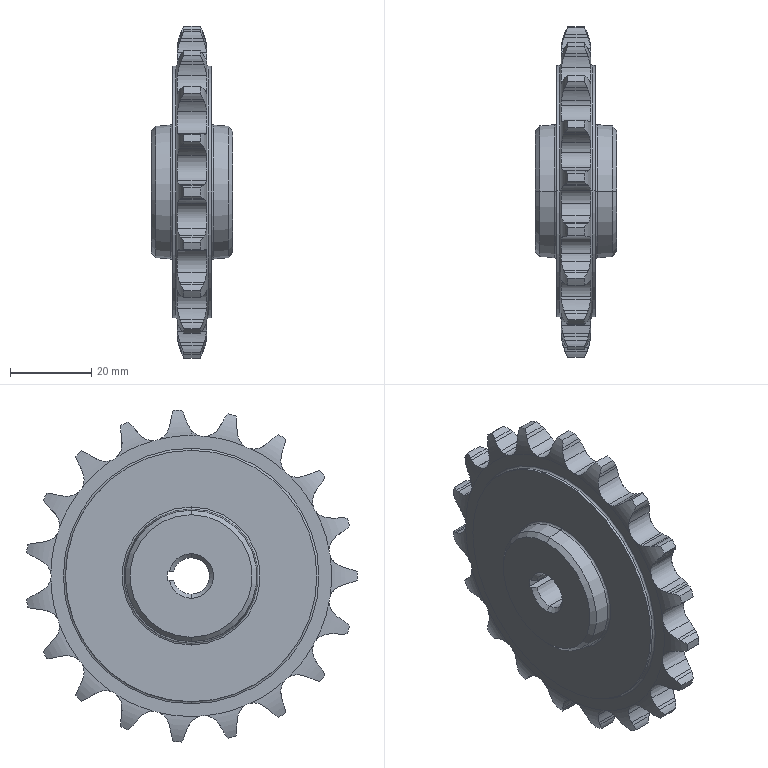Part | SolidWorks | features Cut 2, Revolution 2, Chamfer 1, CirPattern 1, Fillet 1, MirrorPattern 1 | 1 solid | 239 faces | box 20 x 81.595 x 81.862 mm | volume 45176 mm3 | cylinder 130 | torus 48 | plane 47 | cone 14 | commonest cylinder face diameters 11.518 x40 20.732 x40 8.06 x24 82 x19 62 x4 9 x3